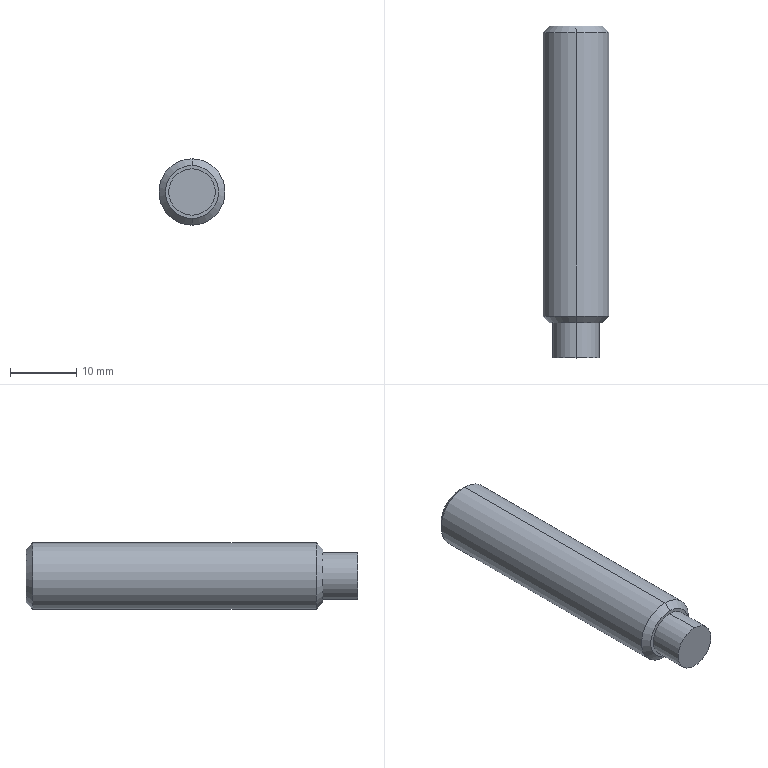Part | SolidWorks | features ICE 3, Chamfer 1, Extrusion 1, RevCut 1 | 1 solid | 31 faces | box 10 x 50 x 10 mm | volume 3601 mm3 | plane 15 | cone 12 | cylinder 4 | commonest cylinder face diameters 7 x2 10 x2
STEP:
#1=CARTESIAN_POINT('',(0.,15.,4.));
#2=VERTEX_POINT('',#1);
#3=CARTESIAN_POINT('',(0.,15.,-4.));
#4=VERTEX_POINT('',#3);
#5=CARTESIAN_POINT('',(0.,15.,0.));
#6=DIRECTION('',(0.,1.,0.));
#7=DIRECTION('',(0.,0.,1.));
#8=AXIS2_PLACEMENT_3D('',#5,#6,#7);
#9=CIRCLE('',#8,4.);
#10=EDGE_CURVE('',#2,#4,#9,.T.);
#11=ORIENTED_EDGE('',*,*,#10,.F.);
#12=CARTESIAN_POINT('',(0.,14.,5.));
#13=VERTEX_POINT('',#12);
#14=CARTESIAN_POINT('',(0.,15.,4.));
#15=DIRECTION('',(0.,-0.7071,0.7071));
#16=VECTOR('',#15,1000.);
#17=LINE('',#14,#16);
#18=EDGE_CURVE('',#2,#13,#17,.T.);
#19=ORIENTED_EDGE('',*,*,#18,.T.);
#20=CARTESIAN_POINT('',(0.,14.,-5.));
#21=VERTEX_POINT('',#20);
#22=CARTESIAN_POINT('',(0.,14.,0.));
#23=DIRECTION('',(0.,-1.,0.));
#24=DIRECTION('',(0.,0.,1.));
#25=AXIS2_PLACEMENT_3D('',#22,#23,#24);
#26=CIRCLE('',#25,5.);
#27=EDGE_CURVE('',#21,#13,#26,.T.);
#28=ORIENTED_EDGE('',*,*,#27,.F.);
#29=CARTESIAN_POINT('',(0.,15.,-4.));
#30=DIRECTION('',(0.,-0.7071,-0.7071));
#31=VECTOR('',#30,1000.);
#32=LINE('',#29,#31);
#33=EDGE_CURVE('',#4,#21,#32,.T.);
#34=ORIENTED_EDGE('',*,*,#33,.F.);
#35=EDGE_LOOP('',(#11,#19,#28,#34));
#36=FACE_OUTER_BOUND('',#35,.T.);
#37=CARTESIAN_POINT('',(0.,15.,0.));
#38=DIRECTION('',(0.,-1.,0.));
#39=DIRECTION('',(0.,0.,-1.));
#40=AXIS2_PLACEMENT_3D('',#37,#38,#39);
#41=CONICAL_SURFACE('',#40,4.,0.7854);
#42=ADVANCED_FACE('',(#36),#41,.T.);
#43=CARTESIAN_POINT('',(0.,-29.7,-4.));
#44=VERTEX_POINT('',#43);
#45=CARTESIAN_POINT('',(0.,-29.7,4.));
#46=VERTEX_POINT('',#45);
#47=CARTESIAN_POINT('',(0.,-29.7,0.));
#48=DIRECTION('',(0.,-1.,0.));
#49=DIRECTION('',(0.,0.,-1.));
#50=AXIS2_PLACEMENT_3D('',#47,#48,#49);
#51=CIRCLE('',#50,4.);
#52=EDGE_CURVE('',#44,#46,#51,.T.);
#53=ORIENTED_EDGE('',*,*,#52,.F.);
#54=CARTESIAN_POINT('',(0.,-28.7,-5.));
#55=VERTEX_POINT('',#54);
#56=CARTESIAN_POINT('',(0.,-29.7,-4.));
#57=DIRECTION('',(0.,0.7071,-0.7071));
#58=VECTOR('',#57,1000.);
#59=LINE('',#56,#58);
#60=EDGE_CURVE('',#44,#55,#59,.T.);
#61=ORIENTED_EDGE('',*,*,#60,.T.);
#62=CARTESIAN_POINT('',(0.,-28.7,5.));
#63=VERTEX_POINT('',#62);
#64=CARTESIAN_POINT('',(0.,-28.7,0.));
#65=DIRECTION('',(0.,1.,0.));
#66=DIRECTION('',(0.,0.,-1.));
#67=AXIS2_PLACEMENT_3D('',#64,#65,#66);
#68=CIRCLE('',#67,5.);
#69=EDGE_CURVE('',#63,#55,#68,.T.);
#70=ORIENTED_EDGE('',*,*,#69,.F.);
#71=CARTESIAN_POINT('',(0.,-29.7,4.));
#72=DIRECTION('',(0.,0.7071,0.7071));
#73=VECTOR('',#72,1000.);
#74=LINE('',#71,#73);
#75=EDGE_CURVE('',#46,#63,#74,.T.);
#76=ORIENTED_EDGE('',*,*,#75,.F.);
#77=EDGE_LOOP('',(#53,#61,#70,#76));
#78=FACE_OUTER_BOUND('',#77,.T.);
#79=CARTESIAN_POINT('',(0.,-29.7,0.));
#80=DIRECTION('',(0.,1.,0.));
#81=DIRECTION('',(0.,0.,1.));
#82=AXIS2_PLACEMENT_3D('',#79,#80,#81);
#83=CONICAL_SURFACE('',#82,4.,0.7854);
#84=ADVANCED_FACE('',(#78),#83,.T.);
#85=CARTESIAN_POINT('',(0.,-29.7,-3.5));
#86=VERTEX_POINT('',#85);
#87=CARTESIAN_POINT('',(0.,-29.7,3.5));
#88=VERTEX_POINT('',#87);
#89=CARTESIAN_POINT('',(0.,-29.7,0.));
#90=DIRECTION('',(0.,-1.,0.));
#91=DIRECTION('',(0.,0.,-1.));
#92=AXIS2_PLACEMENT_3D('',#89,#90,#91);
#93=CIRCLE('',#92,3.5);
#94=EDGE_CURVE('',#86,#88,#93,.T.);
#95=ORIENTED_EDGE('',*,*,#94,.T.);
#96=CARTESIAN_POINT('',(0.,-35.,3.5));
#97=VERTEX_POINT('',#96);
#98=CARTESIAN_POINT('',(0.,-29.7,3.5));
#99=DIRECTION('',(0.,-1.,0.));
#100=VECTOR('',#99,1000.);
#101=LINE('',#98,#100);
#102=EDGE_CURVE('',#88,#97,#101,.T.);
#103=ORIENTED_EDGE('',*,*,#102,.T.);
#104=CARTESIAN_POINT('',(0.,-35.,-3.5));
#105=VERTEX_POINT('',#104);
#106=CARTESIAN_POINT('',(0.,-35.,0.));
#107=DIRECTION('',(0.,-1.,0.));
#108=DIRECTION('',(0.,0.,-1.));
#109=AXIS2_PLACEMENT_3D('',#106,#107,#108);
#110=CIRCLE('',#109,3.5);
#111=EDGE_CURVE('',#105,#97,#110,.T.);
#112=ORIENTED_EDGE('',*,*,#111,.F.);
#113=CARTESIAN_POINT('',(0.,-29.7,-3.5));
#114=DIRECTION('',(0.,-1.,0.));
#115=VECTOR('',#114,1000.);
#116=LINE('',#113,#115);
#117=EDGE_CURVE('',#86,#105,#116,.T.);
#118=ORIENTED_EDGE('',*,*,#117,.F.);
#119=EDGE_LOOP('',(#95,#103,#112,#118));
#120=FACE_OUTER_BOUND('',#119,.T.);
#121=CARTESIAN_POINT('',(0.,-29.7,0.));
#122=DIRECTION('',(0.,-1.,0.));
#123=DIRECTION('',(0.,0.,-1.));
#124=AXIS2_PLACEMENT_3D('',#121,#122,#123);
#125=CYLINDRICAL_SURFACE('',#124,3.5);
#126=ADVANCED_FACE('',(#120),#125,.T.);
#127=CARTESIAN_POINT('',(0.,10.069,0.));
#128=VERTEX_POINT('',#127);
#129=CARTESIAN_POINT('',(0.,11.5,2.478));
#130=VERTEX_POINT('',#129);
#131=CARTESIAN_POINT('',(0.,10.069,0.));
#132=DIRECTION('',(0.,0.5,0.866));
#133=VECTOR('',#132,1000.);
#134=LINE('',#131,#133);
#135=EDGE_CURVE('',#128,#130,#134,.T.);
#136=ORIENTED_EDGE('',*,*,#135,.F.);
#137=CARTESIAN_POINT('',(0.,11.5,-2.478));
#138=VERTEX_POINT('',#137);
#139=CARTESIAN_POINT('',(0.,10.069,0.));
#140=DIRECTION('',(0.,0.5,-0.866));
#141=VECTOR('',#140,1000.);
#142=LINE('',#139,#141);
#143=EDGE_CURVE('',#128,#138,#142,.T.);
#144=ORIENTED_EDGE('',*,*,#143,.T.);
#145=CARTESIAN_POINT('',(-1.239,11.5,-2.146));
#146=VERTEX_POINT('',#145);
#147=CARTESIAN_POINT('',(0.,11.5,0.));
#148=DIRECTION('',(0.,-1.,0.));
#149=DIRECTION('',(0.,0.,-1.));
#150=AXIS2_PLACEMENT_3D('',#147,#148,#149);
#151=CIRCLE('',#150,2.478);
#152=EDGE_CURVE('',#146,#138,#151,.T.);
#153=ORIENTED_EDGE('',*,*,#152,.F.);
#154=CARTESIAN_POINT('',(-2.478,11.5,0.));
#155=VERTEX_POINT('',#154);
#156=CARTESIAN_POINT('',(0.,11.5,0.));
#157=DIRECTION('',(0.,-1.,0.));
#158=DIRECTION('',(0.,0.,-1.));
#159=AXIS2_PLACEMENT_3D('',#156,#157,#158);
#160=CIRCLE('',#159,2.478);
#161=EDGE_CURVE('',#155,#146,#160,.T.);
#162=ORIENTED_EDGE('',*,*,#161,.F.);
#163=CARTESIAN_POINT('',(-1.239,11.5,2.146));
#164=VERTEX_POINT('',#163);
#165=CARTESIAN_POINT('',(0.,11.5,0.));
#166=DIRECTION('',(0.,-1.,0.));
#167=DIRECTION('',(0.,0.,-1.));
#168=AXIS2_PLACEMENT_3D('',#165,#166,#167);
#169=CIRCLE('',#168,2.478);
#170=EDGE_CURVE('',#164,#155,#169,.T.);
#171=ORIENTED_EDGE('',*,*,#170,.F.);
#172=CARTESIAN_POINT('',(0.,11.5,0.));
#173=DIRECTION('',(0.,-1.,0.));
#174=DIRECTION('',(0.,0.,-1.));
#175=AXIS2_PLACEMENT_3D('',#172,#173,#174);
#176=CIRCLE('',#175,2.478);
#177=EDGE_CURVE('',#130,#164,#176,.T.);
#178=ORIENTED_EDGE('',*,*,#177,.F.);
#179=EDGE_LOOP('',(#136,#144,#153,#162,#171,#178));
#180=FACE_OUTER_BOUND('',#179,.T.);
#181=CARTESIAN_POINT('',(0.,1010.069,0.));
#182=DIRECTION('',(0.,1.,0.));
#183=DIRECTION('',(0.,0.,1.));
#184=AXIS2_PLACEMENT_3D('',#181,#182,#183);
#185=CONICAL_SURFACE('',#184,1732.051,1.047);
#186=ADVANCED_FACE('',(#180),#185,.F.);
#187=ORIENTED_EDGE('',*,*,#27,.T.);
#188=CARTESIAN_POINT('',(0.,15.,5.));
#189=DIRECTION('',(0.,-1.,0.));
#190=VECTOR('',#189,1000.);
#191=LINE('',#188,#190);
#192=EDGE_CURVE('',#13,#63,#191,.T.);
#193=ORIENTED_EDGE('',*,*,#192,.T.);
#194=ORIENTED_EDGE('',*,*,#69,.T.);
#195=CARTESIAN_POINT('',(0.,15.,-5.));
#196=DIRECTION('',(0.,-1.,0.));
#197=VECTOR('',#196,1000.);
#198=LINE('',#195,#197);
#199=EDGE_CURVE('',#21,#55,#198,.T.);
#200=ORIENTED_EDGE('',*,*,#199,.F.);
#201=EDGE_LOOP('',(#187,#193,#194,#200));
#202=FACE_OUTER_BOUND('',#201,.T.);
#203=CARTESIAN_POINT('',(0.,15.,0.));
#204=DIRECTION('',(0.,-1.,0.));
#205=DIRECTION('',(0.,0.,-1.));
#206=AXIS2_PLACEMENT_3D('',#203,#204,#205);
#207=CYLINDRICAL_SURFACE('',#206,5.);
#208=ADVANCED_FACE('',(#202),#207,.T.);
#209=ORIENTED_EDGE('',*,*,#192,.F.);
#210=CARTESIAN_POINT('',(0.,14.,0.));
#211=DIRECTION('',(0.,-1.,0.));
#212=DIRECTION('',(0.,0.,1.));
#213=AXIS2_PLACEMENT_3D('',#210,#211,#212);
#214=CIRCLE('',#213,5.);
#215=EDGE_CURVE('',#13,#21,#214,.T.);
#216=ORIENTED_EDGE('',*,*,#215,.T.);
#217=ORIENTED_EDGE('',*,*,#199,.T.);
#218=CARTESIAN_POINT('',(0.,-28.7,0.));
#219=DIRECTION('',(0.,1.,0.));
#220=DIRECTION('',(0.,0.,-1.));
#221=AXIS2_PLACEMENT_3D('',#218,#219,#220);
#222=CIRCLE('',#221,5.);
#223=EDGE_CURVE('',#55,#63,#222,.T.);
#224=ORIENTED_EDGE('',*,*,#223,.T.);
#225=EDGE_LOOP('',(#209,#216,#217,#224));
#226=FACE_OUTER_BOUND('',#225,.T.);
#227=CARTESIAN_POINT('',(0.,15.,0.));
#228=DIRECTION('',(0.,-1.,0.));
#229=DIRECTION('',(0.,0.,-1.));
#230=AXIS2_PLACEMENT_3D('',#227,#228,#229);
#231=CYLINDRICAL_SURFACE('',#230,5.);
#232=ADVANCED_FACE('',(#226),#231,.T.);
#233=CARTESIAN_POINT('',(0.,15.,0.));
#234=DIRECTION('',(0.,1.,0.));
#235=DIRECTION('',(0.,0.,1.));
#236=AXIS2_PLACEMENT_3D('',#233,#234,#235);
#237=CIRCLE('',#236,4.);
#238=EDGE_CURVE('',#4,#2,#237,.T.);
#239=ORIENTED_EDGE('',*,*,#238,.T.);
#240=ORIENTED_EDGE('',*,*,#10,.T.);
#241=EDGE_LOOP('',(#239,#240));
#242=FACE_OUTER_BOUND('',#241,.T.);
#243=CARTESIAN_POINT('',(2.478,15.,1.431));
#244=VERTEX_POINT('',#243);
#245=CARTESIAN_POINT('',(0.,15.,2.862));
#246=VERTEX_POINT('',#245);
#247=CARTESIAN_POINT('',(0.,15.,0.));
#248=DIRECTION('',(0.,-1.,0.));
#249=DIRECTION('',(0.,0.,-1.));
#250=AXIS2_PLACEMENT_3D('',#247,#248,#249);
#251=CIRCLE('',#250,2.861);
#252=EDGE_CURVE('',#244,#246,#251,.T.);
#253=ORIENTED_EDGE('',*,*,#252,.T.);
#254=CARTESIAN_POINT('',(-2.478,15.,1.431));
#255=VERTEX_POINT('',#254);
#256=CARTESIAN_POINT('',(0.,15.,0.));
#257=DIRECTION('',(0.,-1.,0.));
#258=DIRECTION('',(0.,0.,-1.));
#259=AXIS2_PLACEMENT_3D('',#256,#257,#258);
#260=CIRCLE('',#259,2.861);
#261=EDGE_CURVE('',#246,#255,#260,.T.);
#262=ORIENTED_EDGE('',*,*,#261,.T.);
#263=CARTESIAN_POINT('',(-2.478,15.,-1.431));
#264=VERTEX_POINT('',#263);
#265=CARTESIAN_POINT('',(0.,15.,0.));
#266=DIRECTION('',(0.,-1.,0.));
#267=DIRECTION('',(0.,0.,-1.));
#268=AXIS2_PLACEMENT_3D('',#265,#266,#267);
#269=CIRCLE('',#268,2.861);
#270=EDGE_CURVE('',#255,#264,#269,.T.);
#271=ORIENTED_EDGE('',*,*,#270,.T.);
#272=CARTESIAN_POINT('',(0.,15.,-2.861));
#273=VERTEX_POINT('',#272);
#274=CARTESIAN_POINT('',(0.,15.,0.));
#275=DIRECTION('',(0.,-1.,0.));
#276=DIRECTION('',(0.,0.,-1.));
#277=AXIS2_PLACEMENT_3D('',#274,#275,#276);
#278=CIRCLE('',#277,2.861);
#279=EDGE_CURVE('',#264,#273,#278,.T.);
#280=ORIENTED_EDGE('',*,*,#279,.T.);
#281=CARTESIAN_POINT('',(2.478,15.,-1.431));
#282=VERTEX_POINT('',#281);
#283=CARTESIAN_POINT('',(0.,15.,0.));
#284=DIRECTION('',(0.,-1.,0.));
#285=DIRECTION('',(0.,0.,-1.));
#286=AXIS2_PLACEMENT_3D('',#283,#284,#285);
#287=CIRCLE('',#286,2.861);
#288=EDGE_CURVE('',#273,#282,#287,.T.);
#289=ORIENTED_EDGE('',*,*,#288,.T.);
#290=CARTESIAN_POINT('',(0.,15.,0.));
#291=DIRECTION('',(0.,-1.,0.));
#292=DIRECTION('',(0.,0.,-1.));
#293=AXIS2_PLACEMENT_3D('',#290,#291,#292);
#294=CIRCLE('',#293,2.861);
#295=EDGE_CURVE('',#282,#244,#294,.T.);
#296=ORIENTED_EDGE('',*,*,#295,.T.);
#297=EDGE_LOOP('',(#253,#262,#271,#280,#289,#296));
#298=FACE_BOUND('',#297,.T.);
#299=CARTESIAN_POINT('',(0.,15.,0.));
#300=DIRECTION('',(0.,1.,0.));
#301=DIRECTION('',(0.,0.,1.));
#302=AXIS2_PLACEMENT_3D('',#299,#300,#301);
#303=PLANE('',#302);
#304=ADVANCED_FACE('',(#242,#298),#303,.T.);
#305=ORIENTED_EDGE('',*,*,#279,.F.);
#306=CARTESIAN_POINT('',(0.,15.,-2.861));
#307=CARTESIAN_POINT('',(-0.4046,14.865,-2.628));
#308=CARTESIAN_POINT('',(-0.8153,14.779,-2.391));
#309=CARTESIAN_POINT('',(-1.447,14.779,-2.026));
#310=CARTESIAN_POINT('',(-1.658,14.8,-1.904));
#311=CARTESIAN_POINT('',(-2.071,14.877,-1.666));
#312=CARTESIAN_POINT('',(-2.276,14.932,-1.548));
#313=CARTESIAN_POINT('',(-2.478,15.,-1.431));
#314=B_SPLINE_CURVE_WITH_KNOTS('',3,(#306,#307,#308,#309,#310,#311,#312,#313),.UNSPECIFIED.,.F.,.F.,(4,2,2,4),(0.000000238,0.001445,0.002168,0.00289),.UNSPECIFIED.);
#315=EDGE_CURVE('',#273,#264,#314,.T.);
#316=ORIENTED_EDGE('',*,*,#315,.F.);
#317=EDGE_LOOP('',(#305,#316));
#318=FACE_OUTER_BOUND('',#317,.T.);
#319=CARTESIAN_POINT('',(0.,14.779,0.));
#320=DIRECTION('',(0.,1.,0.));
#321=DIRECTION('',(0.,0.,1.));
#322=AXIS2_PLACEMENT_3D('',#319,#320,#321);
#323=CONICAL_SURFACE('',#322,2.478,1.047);
#324=ADVANCED_FACE('',(#318),#323,.F.);
#325=CARTESIAN_POINT('',(-2.478,15.,-1.431));
#326=CARTESIAN_POINT('',(-2.478,14.933,-1.198));
#327=CARTESIAN_POINT('',(-2.478,14.876,-0.9596));
#328=CARTESIAN_POINT('',(-2.478,14.799,-0.4817));
#329=CARTESIAN_POINT('',(-2.478,14.779,-0.2414));
#330=CARTESIAN_POINT('',(-2.478,14.779,0.2423));
#331=CARTESIAN_POINT('',(-2.478,14.8,0.4874));
#332=CARTESIAN_POINT('',(-2.478,14.878,0.9652));
#333=CARTESIAN_POINT('',(-2.478,14.933,1.199));
#334=CARTESIAN_POINT('',(-2.478,15.,1.431));
#335=B_SPLINE_CURVE_WITH_KNOTS('',3,(#325,#326,#327,#328,#329,#330,#331,#332,#333,#334),.UNSPECIFIED.,.F.,.F.,(4,2,2,2,4),(0.002553,0.003277,0.004,0.004724,0.005448),.UNSPECIFIED.);
#336=EDGE_CURVE('',#264,#255,#335,.T.);
#337=ORIENTED_EDGE('',*,*,#336,.F.);
#338=ORIENTED_EDGE('',*,*,#270,.F.);
#339=EDGE_LOOP('',(#337,#338));
#340=FACE_OUTER_BOUND('',#339,.T.);
#341=CARTESIAN_POINT('',(0.,14.779,0.));
#342=DIRECTION('',(0.,1.,0.));
#343=DIRECTION('',(0.,0.,1.));
#344=AXIS2_PLACEMENT_3D('',#341,#342,#343);
#345=CONICAL_SURFACE('',#344,2.478,1.047);
#346=ADVANCED_FACE('',(#340),#345,.F.);
#347=CARTESIAN_POINT('',(-2.478,15.,1.431));
#348=CARTESIAN_POINT('',(-2.074,14.865,1.664));
#349=CARTESIAN_POINT('',(-1.663,14.779,1.901));
#350=CARTESIAN_POINT('',(-1.031,14.779,2.266));
#351=CARTESIAN_POINT('',(-0.8203,14.8,2.388));
#352=CARTESIAN_POINT('',(-0.4068,14.877,2.627));
#353=CARTESIAN_POINT('',(-0.2026,14.932,2.745));
#354=CARTESIAN_POINT('',(0.,15.,2.862));
#355=B_SPLINE_CURVE_WITH_KNOTS('',3,(#347,#348,#349,#350,#351,#352,#353,#354),.UNSPECIFIED.,.F.,.F.,(4,2,2,4),(0.000000238,0.001445,0.002168,0.00289),.UNSPECIFIED.);
#356=EDGE_CURVE('',#255,#246,#355,.T.);
#357=ORIENTED_EDGE('',*,*,#356,.F.);
#358=ORIENTED_EDGE('',*,*,#261,.F.);
#359=EDGE_LOOP('',(#357,#358));
#360=FACE_OUTER_BOUND('',#359,.T.);
#361=CARTESIAN_POINT('',(0.,14.779,0.));
#362=DIRECTION('',(0.,1.,0.));
#363=DIRECTION('',(0.,0.,1.));
#364=AXIS2_PLACEMENT_3D('',#361,#362,#363);
#365=CONICAL_SURFACE('',#364,2.478,1.047);
#366=ADVANCED_FACE('',(#360),#365,.F.);
#367=ORIENTED_EDGE('',*,*,#252,.F.);
#368=CARTESIAN_POINT('',(0.,15.,2.862));
#369=CARTESIAN_POINT('',(0.4046,14.865,2.628));
#370=CARTESIAN_POINT('',(0.8153,14.779,2.391));
#371=CARTESIAN_POINT('',(1.447,14.779,2.026));
#372=CARTESIAN_POINT('',(1.658,14.8,1.904));
#373=CARTESIAN_POINT('',(2.071,14.877,1.666));
#374=CARTESIAN_POINT('',(2.276,14.932,1.548));
#375=CARTESIAN_POINT('',(2.478,15.,1.431));
#376=B_SPLINE_CURVE_WITH_KNOTS('',3,(#368,#369,#370,#371,#372,#373,#374,#375),.UNSPECIFIED.,.F.,.F.,(4,2,2,4),(0.000000238,0.001445,0.002168,0.00289),.UNSPECIFIED.);
#377=EDGE_CURVE('',#246,#244,#376,.T.);
#378=ORIENTED_EDGE('',*,*,#377,.F.);
#379=EDGE_LOOP('',(#367,#378));
#380=FACE_OUTER_BOUND('',#379,.T.);
#381=CARTESIAN_POINT('',(0.,14.779,0.));
#382=DIRECTION('',(0.,1.,0.));
#383=DIRECTION('',(0.,0.,1.));
#384=AXIS2_PLACEMENT_3D('',#381,#382,#383);
#385=CONICAL_SURFACE('',#384,2.478,1.047);
#386=ADVANCED_FACE('',(#380),#385,.F.);
#387=ORIENTED_EDGE('',*,*,#295,.F.);
#388=CARTESIAN_POINT('',(2.478,15.,1.431));
#389=CARTESIAN_POINT('',(2.478,14.933,1.199));
#390=CARTESIAN_POINT('',(2.478,14.878,0.9652));
#391=CARTESIAN_POINT('',(2.478,14.8,0.4874));
#392=CARTESIAN_POINT('',(2.478,14.779,0.2423));
#393=CARTESIAN_POINT('',(2.478,14.779,-0.2414));
#394=CARTESIAN_POINT('',(2.478,14.799,-0.4817));
#395=CARTESIAN_POINT('',(2.478,14.876,-0.9596));
#396=CARTESIAN_POINT('',(2.478,14.933,-1.198));
#397=CARTESIAN_POINT('',(2.478,15.,-1.431));
#398=B_SPLINE_CURVE_WITH_KNOTS('',3,(#388,#389,#390,#391,#392,#393,#394,#395,#396,#397),.UNSPECIFIED.,.F.,.F.,(4,2,2,2,4),(0.001049,0.001771,0.002493,0.003215,0.003937),.UNSPECIFIED.);
#399=EDGE_CURVE('',#244,#282,#398,.T.);
#400=ORIENTED_EDGE('',*,*,#399,.F.);
#401=EDGE_LOOP('',(#387,#400));
#402=FACE_OUTER_BOUND('',#401,.T.);
#403=CARTESIAN_POINT('',(0.,14.779,0.));
#404=DIRECTION('',(0.,1.,0.));
#405=DIRECTION('',(0.,0.,1.));
#406=AXIS2_PLACEMENT_3D('',#403,#404,#405);
#407=CONICAL_SURFACE('',#406,2.478,1.047);
#408=ADVANCED_FACE('',(#402),#407,.F.);
#409=ORIENTED_EDGE('',*,*,#288,.F.);
#410=CARTESIAN_POINT('',(2.478,15.,-1.431));
#411=CARTESIAN_POINT('',(2.074,14.865,-1.664));
#412=CARTESIAN_POINT('',(1.663,14.779,-1.901));
#413=CARTESIAN_POINT('',(1.031,14.779,-2.266));
#414=CARTESIAN_POINT('',(0.8203,14.8,-2.388));
#415=CARTESIAN_POINT('',(0.4068,14.877,-2.627));
#416=CARTESIAN_POINT('',(0.2026,14.932,-2.745));
#417=CARTESIAN_POINT('',(0.,15.,-2.861));
#418=B_SPLINE_CURVE_WITH_KNOTS('',3,(#410,#411,#412,#413,#414,#415,#416,#417),.UNSPECIFIED.,.F.,.F.,(4,2,2,4),(0.000000238,0.001445,0.002168,0.00289),.UNSPECIFIED.);
#419=EDGE_CURVE('',#282,#273,#418,.T.);
#420=ORIENTED_EDGE('',*,*,#419,.F.);
#421=EDGE_LOOP('',(#409,#420));
#422=FACE_OUTER_BOUND('',#421,.T.);
#423=CARTESIAN_POINT('',(0.,14.779,0.));
#424=DIRECTION('',(0.,1.,0.));
#425=DIRECTION('',(0.,0.,1.));
#426=AXIS2_PLACEMENT_3D('',#423,#424,#425);
#427=CONICAL_SURFACE('',#426,2.478,1.047);
#428=ADVANCED_FACE('',(#422),#427,.F.);
#429=ORIENTED_EDGE('',*,*,#143,.F.);
#430=ORIENTED_EDGE('',*,*,#135,.T.);
#431=CARTESIAN_POINT('',(1.239,11.5,2.146));
#432=VERTEX_POINT('',#431);
#433=CARTESIAN_POINT('',(0.,11.5,0.));
#434=DIRECTION('',(0.,-1.,0.));
#435=DIRECTION('',(0.,0.,-1.));
#436=AXIS2_PLACEMENT_3D('',#433,#434,#435);
#437=CIRCLE('',#436,2.478);
#438=EDGE_CURVE('',#432,#130,#437,.T.);
#439=ORIENTED_EDGE('',*,*,#438,.F.);
#440=CARTESIAN_POINT('',(2.478,11.5,0.));
#441=VERTEX_POINT('',#440);
#442=CARTESIAN_POINT('',(0.,11.5,0.));
#443=DIRECTION('',(0.,-1.,0.));
#444=DIRECTION('',(0.,0.,-1.));
#445=AXIS2_PLACEMENT_3D('',#442,#443,#444);
#446=CIRCLE('',#445,2.478);
#447=EDGE_CURVE('',#441,#432,#446,.T.);
#448=ORIENTED_EDGE('',*,*,#447,.F.);
#449=CARTESIAN_POINT('',(1.239,11.5,-2.146));
#450=VERTEX_POINT('',#449);
#451=CARTESIAN_POINT('',(0.,11.5,0.));
#452=DIRECTION('',(0.,-1.,0.));
#453=DIRECTION('',(0.,0.,-1.));
#454=AXIS2_PLACEMENT_3D('',#451,#452,#453);
#455=CIRCLE('',#454,2.478);
#456=EDGE_CURVE('',#450,#441,#455,.T.);
#457=ORIENTED_EDGE('',*,*,#456,.F.);
#458=CARTESIAN_POINT('',(0.,11.5,0.));
#459=DIRECTION('',(0.,-1.,0.));
#460=DIRECTION('',(0.,0.,-1.));
#461=AXIS2_PLACEMENT_3D('',#458,#459,#460);
#462=CIRCLE('',#461,2.478);
#463=EDGE_CURVE('',#138,#450,#462,.T.);
#464=ORIENTED_EDGE('',*,*,#463,.F.);
#465=EDGE_LOOP('',(#429,#430,#439,#448,#457,#464));
#466=FACE_OUTER_BOUND('',#465,.T.);
#467=CARTESIAN_POINT('',(0.,1010.069,0.));
#468=DIRECTION('',(0.,1.,0.));
#469=DIRECTION('',(0.,0.,1.));
#470=AXIS2_PLACEMENT_3D('',#467,#468,#469);
#471=CONICAL_SURFACE('',#470,1732.051,1.047);
#472=ADVANCED_FACE('',(#466),#471,.F.);
#473=CARTESIAN_POINT('',(2.478,11.5,-1.431));
#474=VERTEX_POINT('',#473);
#475=CARTESIAN_POINT('',(2.478,11.5,-1.431));
#476=DIRECTION('',(-0.866,0.,-0.5));
#477=VECTOR('',#476,1000.);
#478=LINE('',#475,#477);
#479=EDGE_CURVE('',#474,#450,#478,.T.);
#480=ORIENTED_EDGE('',*,*,#479,.T.);
#481=ORIENTED_EDGE('',*,*,#456,.T.);
#482=CARTESIAN_POINT('',(2.478,11.5,1.431));
#483=DIRECTION('',(0.,0.,-1.));
#484=VECTOR('',#483,1000.);
#485=LINE('',#482,#484);
#486=EDGE_CURVE('',#441,#474,#485,.T.);
#487=ORIENTED_EDGE('',*,*,#486,.T.);
#488=EDGE_LOOP('',(#480,#481,#487));
#489=FACE_OUTER_BOUND('',#488,.T.);
#490=CARTESIAN_POINT('',(0.,11.5,0.));
#491=DIRECTION('',(0.,1.,0.));
#492=DIRECTION('',(0.,0.,1.));
#493=AXIS2_PLACEMENT_3D('',#490,#491,#492);
#494=PLANE('',#493);
#495=ADVANCED_FACE('',(#489),#494,.T.);
#496=CARTESIAN_POINT('',(2.478,11.5,1.431));
#497=VERTEX_POINT('',#496);
#498=CARTESIAN_POINT('',(2.478,11.5,1.431));
#499=DIRECTION('',(0.,0.,-1.));
#500=VECTOR('',#499,1000.);
#501=LINE('',#498,#500);
#502=EDGE_CURVE('',#497,#441,#501,.T.);
#503=ORIENTED_EDGE('',*,*,#502,.T.);
#504=ORIENTED_EDGE('',*,*,#447,.T.);
#505=CARTESIAN_POINT('',(0.,11.5,2.862));
#506=DIRECTION('',(0.866,0.,-0.5));
#507=VECTOR('',#506,1000.);
#508=LINE('',#505,#507);
#509=EDGE_CURVE('',#432,#497,#508,.T.);
#510=ORIENTED_EDGE('',*,*,#509,.T.);
#511=EDGE_LOOP('',(#503,#504,#510));
#512=FACE_OUTER_BOUND('',#511,.T.);
#513=CARTESIAN_POINT('',(0.,11.5,0.));
#514=DIRECTION('',(0.,1.,0.));
#515=DIRECTION('',(0.,0.,1.));
#516=AXIS2_PLACEMENT_3D('',#513,#514,#515);
#517=PLANE('',#516);
#518=ADVANCED_FACE('',(#512),#517,.T.);
#519=CARTESIAN_POINT('',(0.,11.5,2.862));
#520=VERTEX_POINT('',#519);
#521=CARTESIAN_POINT('',(0.,11.5,2.862));
#522=DIRECTION('',(0.866,0.,-0.5));
#523=VECTOR('',#522,1000.);
#524=LINE('',#521,#523);
#525=EDGE_CURVE('',#520,#432,#524,.T.);
#526=ORIENTED_EDGE('',*,*,#525,.T.);
#527=ORIENTED_EDGE('',*,*,#438,.T.);
#528=ORIENTED_EDGE('',*,*,#177,.T.);
#529=CARTESIAN_POINT('',(-2.478,11.5,1.431));
#530=DIRECTION('',(0.866,0.,0.5));
#531=VECTOR('',#530,1000.);
#532=LINE('',#529,#531);
#533=EDGE_CURVE('',#164,#520,#532,.T.);
#534=ORIENTED_EDGE('',*,*,#533,.T.);
#535=EDGE_LOOP('',(#526,#527,#528,#534));
#536=FACE_OUTER_BOUND('',#535,.T.);
#537=CARTESIAN_POINT('',(0.,11.5,0.));
#538=DIRECTION('',(0.,1.,0.));
#539=DIRECTION('',(0.,0.,1.));
#540=AXIS2_PLACEMENT_3D('',#537,#538,#539);
#541=PLANE('',#540);
#542=ADVANCED_FACE('',(#536),#541,.T.);
#543=CARTESIAN_POINT('',(-2.478,11.5,1.431));
#544=VERTEX_POINT('',#543);
#545=CARTESIAN_POINT('',(-2.478,11.5,1.431));
#546=DIRECTION('',(0.866,0.,0.5));
#547=VECTOR('',#546,1000.);
#548=LINE('',#545,#547);
#549=EDGE_CURVE('',#544,#164,#548,.T.);
#550=ORIENTED_EDGE('',*,*,#549,.T.);
#551=ORIENTED_EDGE('',*,*,#170,.T.);
#552=CARTESIAN_POINT('',(-2.478,11.5,-1.431));
#553=DIRECTION('',(0.,0.,1.));
#554=VECTOR('',#553,1000.);
#555=LINE('',#552,#554);
#556=EDGE_CURVE('',#155,#544,#555,.T.);
#557=ORIENTED_EDGE('',*,*,#556,.T.);
#558=EDGE_LOOP('',(#550,#551,#557));
#559=FACE_OUTER_BOUND('',#558,.T.);
#560=CARTESIAN_POINT('',(0.,11.5,0.));
#561=DIRECTION('',(0.,1.,0.));
#562=DIRECTION('',(0.,0.,1.));
#563=AXIS2_PLACEMENT_3D('',#560,#561,#562);
#564=PLANE('',#563);
#565=ADVANCED_FACE('',(#559),#564,.T.);
#566=CARTESIAN_POINT('',(0.,11.5,-2.861));
#567=VERTEX_POINT('',#566);
#568=CARTESIAN_POINT('',(0.,11.5,-2.861));
#569=DIRECTION('',(-0.866,0.,0.5));
#570=VECTOR('',#569,1000.);
#571=LINE('',#568,#570);
#572=EDGE_CURVE('',#567,#146,#571,.T.);
#573=ORIENTED_EDGE('',*,*,#572,.T.);
#574=ORIENTED_EDGE('',*,*,#152,.T.);
#575=ORIENTED_EDGE('',*,*,#463,.T.);
#576=CARTESIAN_POINT('',(2.478,11.5,-1.431));
#577=DIRECTION('',(-0.866,0.,-0.5));
#578=VECTOR('',#577,1000.);
#579=LINE('',#576,#578);
#580=EDGE_CURVE('',#450,#567,#579,.T.);
#581=ORIENTED_EDGE('',*,*,#580,.T.);
#582=EDGE_LOOP('',(#573,#574,#575,#581));
#583=FACE_OUTER_BOUND('',#582,.T.);
#584=CARTESIAN_POINT('',(0.,11.5,0.));
#585=DIRECTION('',(0.,1.,0.));
#586=DIRECTION('',(0.,0.,1.));
#587=AXIS2_PLACEMENT_3D('',#584,#585,#586);
#588=PLANE('',#587);
#589=ADVANCED_FACE('',(#583),#588,.T.);
#590=CARTESIAN_POINT('',(-2.478,11.5,-1.431));
#591=VERTEX_POINT('',#590);
#592=CARTESIAN_POINT('',(-2.478,11.5,-1.431));
#593=DIRECTION('',(0.,0.,1.));
#594=VECTOR('',#593,1000.);
#595=LINE('',#592,#594);
#596=EDGE_CURVE('',#591,#155,#595,.T.);
#597=ORIENTED_EDGE('',*,*,#596,.T.);
#598=ORIENTED_EDGE('',*,*,#161,.T.);
#599=CARTESIAN_POINT('',(0.,11.5,-2.861));
#600=DIRECTION('',(-0.866,0.,0.5));
#601=VECTOR('',#600,1000.);
#602=LINE('',#599,#601);
#603=EDGE_CURVE('',#146,#591,#602,.T.);
#604=ORIENTED_EDGE('',*,*,#603,.T.);
#605=EDGE_LOOP('',(#597,#598,#604));
#606=FACE_OUTER_BOUND('',#605,.T.);
#607=CARTESIAN_POINT('',(0.,11.5,0.));
#608=DIRECTION('',(0.,1.,0.));
#609=DIRECTION('',(0.,0.,1.));
#610=AXIS2_PLACEMENT_3D('',#607,#608,#609);
#611=PLANE('',#610);
#612=ADVANCED_FACE('',(#606),#611,.T.);
#613=CARTESIAN_POINT('',(0.,11.5,-2.861));
#614=DIRECTION('',(0.,1.,0.));
#615=VECTOR('',#614,1000.);
#616=LINE('',#613,#615);
#617=EDGE_CURVE('',#567,#273,#616,.T.);
#618=ORIENTED_EDGE('',*,*,#617,.T.);
#619=ORIENTED_EDGE('',*,*,#315,.T.);
#620=CARTESIAN_POINT('',(-2.478,11.5,-1.431));
#621=DIRECTION('',(0.,1.,0.));
#622=VECTOR('',#621,1000.);
#623=LINE('',#620,#622);
#624=EDGE_CURVE('',#591,#264,#623,.T.);
#625=ORIENTED_EDGE('',*,*,#624,.F.);
#626=ORIENTED_EDGE('',*,*,#603,.F.);
#627=ORIENTED_EDGE('',*,*,#572,.F.);
#628=EDGE_LOOP('',(#618,#619,#625,#626,#627));
#629=FACE_OUTER_BOUND('',#628,.T.);
#630=CARTESIAN_POINT('',(0.,11.5,-2.861));
#631=DIRECTION('',(-0.5,0.,-0.866));
#632=DIRECTION('',(-0.866,0.,0.5));
#633=AXIS2_PLACEMENT_3D('',#630,#631,#632);
#634=PLANE('',#633);
#635=ADVANCED_FACE('',(#629),#634,.F.);
#636=ORIENTED_EDGE('',*,*,#624,.T.);
#637=ORIENTED_EDGE('',*,*,#336,.T.);
#638=CARTESIAN_POINT('',(-2.478,11.5,1.431));
#639=DIRECTION('',(0.,1.,0.));
#640=VECTOR('',#639,1000.);
#641=LINE('',#638,#640);
#642=EDGE_CURVE('',#544,#255,#641,.T.);
#643=ORIENTED_EDGE('',*,*,#642,.F.);
#644=ORIENTED_EDGE('',*,*,#556,.F.);
#645=ORIENTED_EDGE('',*,*,#596,.F.);
#646=EDGE_LOOP('',(#636,#637,#643,#644,#645));
#647=FACE_OUTER_BOUND('',#646,.T.);
#648=CARTESIAN_POINT('',(-2.478,11.5,-1.431));
#649=DIRECTION('',(-1.,0.,0.));
#650=DIRECTION('',(0.,0.,1.));
#651=AXIS2_PLACEMENT_3D('',#648,#649,#650);
#652=PLANE('',#651);
#653=ADVANCED_FACE('',(#647),#652,.F.);
#654=ORIENTED_EDGE('',*,*,#642,.T.);
#655=ORIENTED_EDGE('',*,*,#356,.T.);
#656=CARTESIAN_POINT('',(0.,11.5,2.862));
#657=DIRECTION('',(0.,1.,0.));
#658=VECTOR('',#657,1000.);
#659=LINE('',#656,#658);
#660=EDGE_CURVE('',#520,#246,#659,.T.);
#661=ORIENTED_EDGE('',*,*,#660,.F.);
#662=ORIENTED_EDGE('',*,*,#533,.F.);
#663=ORIENTED_EDGE('',*,*,#549,.F.);
#664=EDGE_LOOP('',(#654,#655,#661,#662,#663));
#665=FACE_OUTER_BOUND('',#664,.T.);
#666=CARTESIAN_POINT('',(-2.478,11.5,1.431));
#667=DIRECTION('',(-0.5,0.,0.866));
#668=DIRECTION('',(0.866,0.,0.5));
#669=AXIS2_PLACEMENT_3D('',#666,#667,#668);
#670=PLANE('',#669);
#671=ADVANCED_FACE('',(#665),#670,.F.);
#672=ORIENTED_EDGE('',*,*,#660,.T.);
#673=ORIENTED_EDGE('',*,*,#377,.T.);
#674=CARTESIAN_POINT('',(2.478,11.5,1.431));
#675=DIRECTION('',(0.,1.,0.));
#676=VECTOR('',#675,1000.);
#677=LINE('',#674,#676);
#678=EDGE_CURVE('',#497,#244,#677,.T.);
#679=ORIENTED_EDGE('',*,*,#678,.F.);
#680=ORIENTED_EDGE('',*,*,#509,.F.);
#681=ORIENTED_EDGE('',*,*,#525,.F.);
#682=EDGE_LOOP('',(#672,#673,#679,#680,#681));
#683=FACE_OUTER_BOUND('',#682,.T.);
#684=CARTESIAN_POINT('',(0.,11.5,2.862));
#685=DIRECTION('',(0.5,0.,0.866));
#686=DIRECTION('',(0.866,0.,-0.5));
#687=AXIS2_PLACEMENT_3D('',#684,#685,#686);
#688=PLANE('',#687);
#689=ADVANCED_FACE('',(#683),#688,.F.);
#690=ORIENTED_EDGE('',*,*,#678,.T.);
#691=ORIENTED_EDGE('',*,*,#399,.T.);
#692=CARTESIAN_POINT('',(2.478,11.5,-1.431));
#693=DIRECTION('',(0.,1.,0.));
#694=VECTOR('',#693,1000.);
#695=LINE('',#692,#694);
#696=EDGE_CURVE('',#474,#282,#695,.T.);
#697=ORIENTED_EDGE('',*,*,#696,.F.);
#698=ORIENTED_EDGE('',*,*,#486,.F.);
#699=ORIENTED_EDGE('',*,*,#502,.F.);
#700=EDGE_LOOP('',(#690,#691,#697,#698,#699));
#701=FACE_OUTER_BOUND('',#700,.T.);
#702=CARTESIAN_POINT('',(2.478,11.5,1.431));
#703=DIRECTION('',(1.,0.,0.));
#704=DIRECTION('',(0.,0.,-1.));
#705=AXIS2_PLACEMENT_3D('',#702,#703,#704);
#706=PLANE('',#705);
#707=ADVANCED_FACE('',(#701),#706,.F.);
#708=ORIENTED_EDGE('',*,*,#696,.T.);
#709=ORIENTED_EDGE('',*,*,#419,.T.);
#710=ORIENTED_EDGE('',*,*,#617,.F.);
#711=ORIENTED_EDGE('',*,*,#580,.F.);
#712=ORIENTED_EDGE('',*,*,#479,.F.);
#713=EDGE_LOOP('',(#708,#709,#710,#711,#712));
#714=FACE_OUTER_BOUND('',#713,.T.);
#715=CARTESIAN_POINT('',(2.478,11.5,-1.431));
#716=DIRECTION('',(0.5,0.,-0.866));
#717=DIRECTION('',(-0.866,0.,-0.5));
#718=AXIS2_PLACEMENT_3D('',#715,#716,#717);
#719=PLANE('',#718);
#720=ADVANCED_FACE('',(#714),#719,.F.);
#721=CARTESIAN_POINT('',(0.,-29.7,0.));
#722=DIRECTION('',(0.,-1.,0.));
#723=DIRECTION('',(0.,0.,-1.));
#724=AXIS2_PLACEMENT_3D('',#721,#722,#723);
#725=CIRCLE('',#724,4.);
#726=EDGE_CURVE('',#46,#44,#725,.T.);
#727=ORIENTED_EDGE('',*,*,#726,.T.);
#728=ORIENTED_EDGE('',*,*,#52,.T.);
#729=EDGE_LOOP('',(#727,#728));
#730=FACE_OUTER_BOUND('',#729,.T.);
#731=ORIENTED_EDGE('',*,*,#94,.F.);
#732=CARTESIAN_POINT('',(0.,-29.7,0.));
#733=DIRECTION('',(0.,-1.,0.));
#734=DIRECTION('',(0.,0.,-1.));
#735=AXIS2_PLACEMENT_3D('',#732,#733,#734);
#736=CIRCLE('',#735,3.5);
#737=EDGE_CURVE('',#88,#86,#736,.T.);
#738=ORIENTED_EDGE('',*,*,#737,.F.);
#739=EDGE_LOOP('',(#731,#738));
#740=FACE_BOUND('',#739,.T.);
#741=CARTESIAN_POINT('',(0.,-29.7,0.));
#742=DIRECTION('',(0.,-1.,0.));
#743=DIRECTION('',(0.,0.,-1.));
#744=AXIS2_PLACEMENT_3D('',#741,#742,#743);
#745=PLANE('',#744);
#746=ADVANCED_FACE('',(#730,#740),#745,.T.);
#747=ORIENTED_EDGE('',*,*,#102,.F.);
#748=ORIENTED_EDGE('',*,*,#737,.T.);
#749=ORIENTED_EDGE('',*,*,#117,.T.);
#750=CARTESIAN_POINT('',(0.,-35.,0.));
#751=DIRECTION('',(0.,-1.,0.));
#752=DIRECTION('',(0.,0.,-1.));
#753=AXIS2_PLACEMENT_3D('',#750,#751,#752);
#754=CIRCLE('',#753,3.5);
#755=EDGE_CURVE('',#97,#105,#754,.T.);
#756=ORIENTED_EDGE('',*,*,#755,.F.);
#757=EDGE_LOOP('',(#747,#748,#749,#756));
#758=FACE_OUTER_BOUND('',#757,.T.);
#759=CARTESIAN_POINT('',(0.,-29.7,0.));
#760=DIRECTION('',(0.,-1.,0.));
#761=DIRECTION('',(0.,0.,-1.));
#762=AXIS2_PLACEMENT_3D('',#759,#760,#761);
#763=CYLINDRICAL_SURFACE('',#762,3.5);
#764=ADVANCED_FACE('',(#758),#763,.T.);
#765=ORIENTED_EDGE('',*,*,#111,.T.);
#766=ORIENTED_EDGE('',*,*,#755,.T.);
#767=EDGE_LOOP('',(#765,#766));
#768=FACE_OUTER_BOUND('',#767,.T.);
#769=CARTESIAN_POINT('',(0.,-35.,0.));
#770=DIRECTION('',(0.,-1.,0.));
#771=DIRECTION('',(0.,0.,-1.));
#772=AXIS2_PLACEMENT_3D('',#769,#770,#771);
#773=PLANE('',#772);
#774=ADVANCED_FACE('',(#768),#773,.T.);
#775=ORIENTED_EDGE('',*,*,#60,.F.);
#776=ORIENTED_EDGE('',*,*,#726,.F.);
#777=ORIENTED_EDGE('',*,*,#75,.T.);
#778=ORIENTED_EDGE('',*,*,#223,.F.);
#779=EDGE_LOOP('',(#775,#776,#777,#778));
#780=FACE_OUTER_BOUND('',#779,.T.);
#781=CARTESIAN_POINT('',(0.,-29.7,0.));
#782=DIRECTION('',(0.,1.,0.));
#783=DIRECTION('',(0.,0.,1.));
#784=AXIS2_PLACEMENT_3D('',#781,#782,#783);
#785=CONICAL_SURFACE('',#784,4.,0.7854);
#786=ADVANCED_FACE('',(#780),#785,.T.);
#787=ORIENTED_EDGE('',*,*,#18,.F.);
#788=ORIENTED_EDGE('',*,*,#238,.F.);
#789=ORIENTED_EDGE('',*,*,#33,.T.);
#790=ORIENTED_EDGE('',*,*,#215,.F.);
#791=EDGE_LOOP('',(#787,#788,#789,#790));
#792=FACE_OUTER_BOUND('',#791,.T.);
#793=CARTESIAN_POINT('',(0.,15.,0.));
#794=DIRECTION('',(0.,-1.,0.));
#795=DIRECTION('',(0.,0.,-1.));
#796=AXIS2_PLACEMENT_3D('',#793,#794,#795);
#797=CONICAL_SURFACE('',#796,4.,0.7854);
#798=ADVANCED_FACE('',(#792),#797,.T.);
#799=CLOSED_SHELL('',(#42,#84,#126,#186,#208,#232,#304,#324,#346,#366,#386,#408,#428,#472,#495,#518,#542,#565,#589,#612,#635,#653,#671,#689,#707,#720,#746,#764,#774,#786,#798));
#800=MANIFOLD_SOLID_BREP('',#799);
#801=CARTESIAN_POINT('',(0.,0.,0.));
#802=DIRECTION('',(0.,0.,1.));
#803=DIRECTION('',(1.,0.,0.));
#804=AXIS2_PLACEMENT_3D('',#801,#802,#803);
#805=(LENGTH_UNIT()NAMED_UNIT(*)SI_UNIT(.MILLI.,.METRE.));
#806=UNCERTAINTY_MEASURE_WITH_UNIT(LENGTH_MEASURE(0.00001),#805,'','');
#807=(NAMED_UNIT(*)PLANE_ANGLE_UNIT()SI_UNIT($,.RADIAN.));
#808=(NAMED_UNIT(*)SI_UNIT($,.STERADIAN.)SOLID_ANGLE_UNIT());
#809=(GEOMETRIC_REPRESENTATION_CONTEXT(3)GLOBAL_UNCERTAINTY_ASSIGNED_CONTEXT((#806))GLOBAL_UNIT_ASSIGNED_CONTEXT((#805,#807,#808))REPRESENTATION_CONTEXT('',''));
#810=ADVANCED_BREP_SHAPE_REPRESENTATION('',(#800,#804),#809);